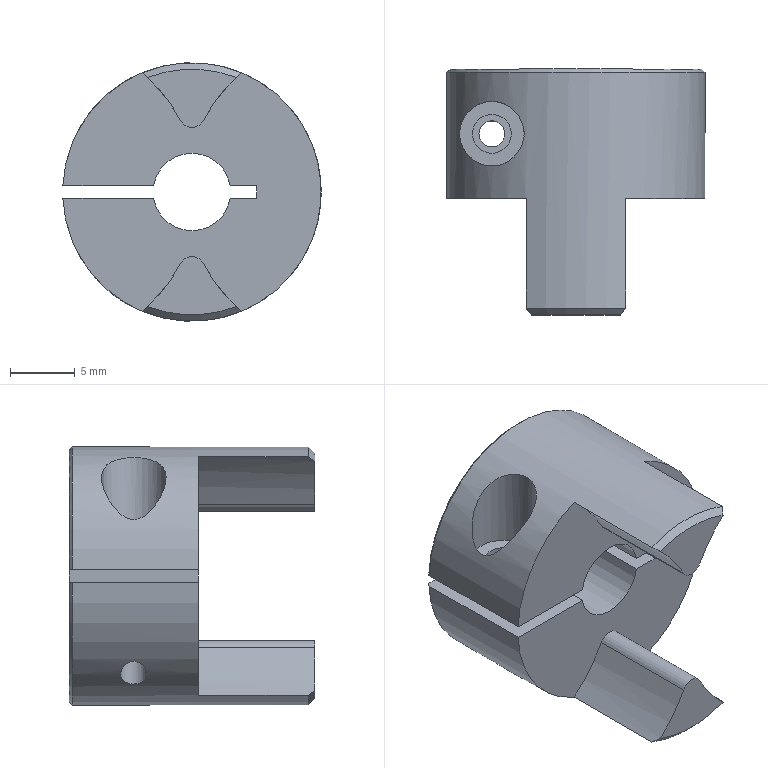Part | NX | features L-HUB_5003_022_GCJC20-BL-6-8 2 | 1 solid | 25 faces | box 19.987 x 19 x 20 mm | volume 3007 mm3 | cylinder 12 | plane 10 | cone 3 | commonest cylinder face diameters 24 x4 2 x2 6 x2 2.013 x1 3 x1 5 x1
STEP:
#1=CARTESIAN_POINT('',(-226.762,-568.6,-110.));
#2=VERTEX_POINT('',#1);
#3=CARTESIAN_POINT('',(-219.733,-568.6,-110.));
#4=VERTEX_POINT('',#3);
#5=CARTESIAN_POINT('',(-211.775,-568.6,-110.));
#6=DIRECTION('',(1.,0.,0.));
#7=VECTOR('',#6,1000.);
#8=LINE('',#5,#7);
#9=EDGE_CURVE('',#2,#4,#8,.T.);
#10=ORIENTED_EDGE('',*,*,#9,.T.);
#11=CARTESIAN_POINT('',(-213.817,-568.6,-110.));
#12=VERTEX_POINT('',#11);
#13=CARTESIAN_POINT('',(-216.775,-568.6,-110.5));
#14=DIRECTION('',(0.,1.,0.));
#15=DIRECTION('',(-1.,0.,0.));
#16=AXIS2_PLACEMENT_3D('',#13,#14,#15);
#17=CIRCLE('',#16,3.);
#18=EDGE_CURVE('',#4,#12,#17,.T.);
#19=ORIENTED_EDGE('',*,*,#18,.T.);
#20=CARTESIAN_POINT('',(-211.775,-568.6,-110.));
#21=VERTEX_POINT('',#20);
#22=CARTESIAN_POINT('',(-211.775,-568.6,-110.));
#23=DIRECTION('',(1.,0.,0.));
#24=VECTOR('',#23,1000.);
#25=LINE('',#22,#24);
#26=EDGE_CURVE('',#12,#21,#25,.T.);
#27=ORIENTED_EDGE('',*,*,#26,.T.);
#28=CARTESIAN_POINT('',(-211.775,-568.6,-111.));
#29=VERTEX_POINT('',#28);
#30=CARTESIAN_POINT('',(-211.775,-568.6,-111.));
#31=DIRECTION('',(0.,0.,-1.));
#32=VECTOR('',#31,1000.);
#33=LINE('',#30,#32);
#34=EDGE_CURVE('',#21,#29,#33,.T.);
#35=ORIENTED_EDGE('',*,*,#34,.T.);
#36=CARTESIAN_POINT('',(-213.817,-568.6,-111.));
#37=VERTEX_POINT('',#36);
#38=CARTESIAN_POINT('',(-226.762,-568.6,-111.));
#39=DIRECTION('',(-1.,0.,0.));
#40=VECTOR('',#39,1000.);
#41=LINE('',#38,#40);
#42=EDGE_CURVE('',#29,#37,#41,.T.);
#43=ORIENTED_EDGE('',*,*,#42,.T.);
#44=CARTESIAN_POINT('',(-219.733,-568.6,-111.));
#45=VERTEX_POINT('',#44);
#46=CARTESIAN_POINT('',(-216.775,-568.6,-110.5));
#47=DIRECTION('',(0.,1.,0.));
#48=DIRECTION('',(-1.,0.,0.));
#49=AXIS2_PLACEMENT_3D('',#46,#47,#48);
#50=CIRCLE('',#49,3.);
#51=EDGE_CURVE('',#37,#45,#50,.T.);
#52=ORIENTED_EDGE('',*,*,#51,.T.);
#53=CARTESIAN_POINT('',(-226.762,-568.6,-111.));
#54=VERTEX_POINT('',#53);
#55=CARTESIAN_POINT('',(-226.762,-568.6,-111.));
#56=DIRECTION('',(-1.,0.,0.));
#57=VECTOR('',#56,1000.);
#58=LINE('',#55,#57);
#59=EDGE_CURVE('',#45,#54,#58,.T.);
#60=ORIENTED_EDGE('',*,*,#59,.T.);
#61=CARTESIAN_POINT('',(-220.634,-568.6,-119.726));
#62=VERTEX_POINT('',#61);
#63=CARTESIAN_POINT('',(-216.775,-568.6,-110.5));
#64=DIRECTION('',(0.,1.,0.));
#65=DIRECTION('',(-1.,0.,0.));
#66=AXIS2_PLACEMENT_3D('',#63,#64,#65);
#67=CIRCLE('',#66,10.);
#68=EDGE_CURVE('',#62,#54,#67,.T.);
#69=ORIENTED_EDGE('',*,*,#68,.F.);
#70=CARTESIAN_POINT('',(-217.662,-568.6,-116.038));
#71=VERTEX_POINT('',#70);
#72=CARTESIAN_POINT('',(-228.308,-568.6,-110.5));
#73=DIRECTION('',(0.,1.,0.));
#74=DIRECTION('',(1.,0.,0.));
#75=AXIS2_PLACEMENT_3D('',#72,#73,#74);
#76=CIRCLE('',#75,12.);
#77=EDGE_CURVE('',#71,#62,#76,.T.);
#78=ORIENTED_EDGE('',*,*,#77,.F.);
#79=CARTESIAN_POINT('',(-215.888,-568.6,-116.038));
#80=VERTEX_POINT('',#79);
#81=CARTESIAN_POINT('',(-216.775,-568.6,-116.5));
#82=DIRECTION('',(0.,-1.,0.));
#83=DIRECTION('',(1.,0.,0.));
#84=AXIS2_PLACEMENT_3D('',#81,#82,#83);
#85=CIRCLE('',#84,1.);
#86=EDGE_CURVE('',#80,#71,#85,.T.);
#87=ORIENTED_EDGE('',*,*,#86,.F.);
#88=CARTESIAN_POINT('',(-212.916,-568.6,-119.726));
#89=VERTEX_POINT('',#88);
#90=CARTESIAN_POINT('',(-205.242,-568.6,-110.5));
#91=DIRECTION('',(0.,1.,0.));
#92=DIRECTION('',(1.,0.,0.));
#93=AXIS2_PLACEMENT_3D('',#90,#91,#92);
#94=CIRCLE('',#93,12.);
#95=EDGE_CURVE('',#89,#80,#94,.T.);
#96=ORIENTED_EDGE('',*,*,#95,.F.);
#97=CARTESIAN_POINT('',(-212.916,-568.6,-101.274));
#98=VERTEX_POINT('',#97);
#99=CARTESIAN_POINT('',(-216.775,-568.6,-110.5));
#100=DIRECTION('',(0.,1.,0.));
#101=DIRECTION('',(-1.,0.,0.));
#102=AXIS2_PLACEMENT_3D('',#99,#100,#101);
#103=CIRCLE('',#102,10.);
#104=EDGE_CURVE('',#98,#89,#103,.T.);
#105=ORIENTED_EDGE('',*,*,#104,.F.);
#106=CARTESIAN_POINT('',(-215.888,-568.6,-104.962));
#107=VERTEX_POINT('',#106);
#108=CARTESIAN_POINT('',(-205.242,-568.6,-110.5));
#109=DIRECTION('',(0.,1.,0.));
#110=DIRECTION('',(1.,0.,0.));
#111=AXIS2_PLACEMENT_3D('',#108,#109,#110);
#112=CIRCLE('',#111,12.);
#113=EDGE_CURVE('',#107,#98,#112,.T.);
#114=ORIENTED_EDGE('',*,*,#113,.F.);
#115=CARTESIAN_POINT('',(-217.662,-568.6,-104.962));
#116=VERTEX_POINT('',#115);
#117=CARTESIAN_POINT('',(-216.775,-568.6,-104.5));
#118=DIRECTION('',(0.,-1.,0.));
#119=DIRECTION('',(1.,0.,0.));
#120=AXIS2_PLACEMENT_3D('',#117,#118,#119);
#121=CIRCLE('',#120,1.);
#122=EDGE_CURVE('',#116,#107,#121,.T.);
#123=ORIENTED_EDGE('',*,*,#122,.F.);
#124=CARTESIAN_POINT('',(-220.634,-568.6,-101.274));
#125=VERTEX_POINT('',#124);
#126=CARTESIAN_POINT('',(-228.308,-568.6,-110.5));
#127=DIRECTION('',(0.,1.,0.));
#128=DIRECTION('',(1.,0.,0.));
#129=AXIS2_PLACEMENT_3D('',#126,#127,#128);
#130=CIRCLE('',#129,12.);
#131=EDGE_CURVE('',#125,#116,#130,.T.);
#132=ORIENTED_EDGE('',*,*,#131,.F.);
#133=CARTESIAN_POINT('',(-216.775,-568.6,-110.5));
#134=DIRECTION('',(0.,1.,0.));
#135=DIRECTION('',(-1.,0.,0.));
#136=AXIS2_PLACEMENT_3D('',#133,#134,#135);
#137=CIRCLE('',#136,10.);
#138=EDGE_CURVE('',#2,#125,#137,.T.);
#139=ORIENTED_EDGE('',*,*,#138,.F.);
#140=EDGE_LOOP('',(#10,#19,#27,#35,#43,#52,#60,#69,#78,#87,#96,#105,#114,#123,#132,#139));
#141=FACE_BOUND('',#140,.T.);
#142=CARTESIAN_POINT('',(-216.775,-568.6,-110.5));
#143=DIRECTION('',(0.,1.,0.));
#144=DIRECTION('',(-1.,0.,0.));
#145=AXIS2_PLACEMENT_3D('',#142,#143,#144);
#146=PLANE('',#145);
#147=ADVANCED_FACE('',(#141),#146,.F.);
#148=CARTESIAN_POINT('',(-219.733,-558.6,-110.));
#149=VERTEX_POINT('',#148);
#150=CARTESIAN_POINT('',(-226.512,-558.6,-110.));
#151=VERTEX_POINT('',#150);
#152=CARTESIAN_POINT('',(-211.775,-558.6,-110.));
#153=DIRECTION('',(-1.,0.,0.));
#154=VECTOR('',#153,1000.);
#155=LINE('',#152,#154);
#156=EDGE_CURVE('',#149,#151,#155,.T.);
#157=ORIENTED_EDGE('',*,*,#156,.T.);
#158=CARTESIAN_POINT('',(-226.512,-558.6,-111.));
#159=VERTEX_POINT('',#158);
#160=CARTESIAN_POINT('',(-216.775,-558.6,-110.5));
#161=DIRECTION('',(0.,-1.,0.));
#162=DIRECTION('',(1.,0.,0.));
#163=AXIS2_PLACEMENT_3D('',#160,#161,#162);
#164=CIRCLE('',#163,9.75);
#165=EDGE_CURVE('',#151,#159,#164,.F.);
#166=ORIENTED_EDGE('',*,*,#165,.T.);
#167=CARTESIAN_POINT('',(-219.733,-558.6,-111.));
#168=VERTEX_POINT('',#167);
#169=CARTESIAN_POINT('',(-226.762,-558.6,-111.));
#170=DIRECTION('',(1.,0.,0.));
#171=VECTOR('',#170,1000.);
#172=LINE('',#169,#171);
#173=EDGE_CURVE('',#159,#168,#172,.T.);
#174=ORIENTED_EDGE('',*,*,#173,.T.);
#175=CARTESIAN_POINT('',(-213.817,-558.6,-111.));
#176=VERTEX_POINT('',#175);
#177=CARTESIAN_POINT('',(-216.775,-558.6,-110.5));
#178=DIRECTION('',(0.,-1.,0.));
#179=DIRECTION('',(1.,0.,0.));
#180=AXIS2_PLACEMENT_3D('',#177,#178,#179);
#181=CIRCLE('',#180,3.);
#182=EDGE_CURVE('',#168,#176,#181,.T.);
#183=ORIENTED_EDGE('',*,*,#182,.T.);
#184=CARTESIAN_POINT('',(-211.775,-558.6,-111.));
#185=VERTEX_POINT('',#184);
#186=CARTESIAN_POINT('',(-226.762,-558.6,-111.));
#187=DIRECTION('',(1.,0.,0.));
#188=VECTOR('',#187,1000.);
#189=LINE('',#186,#188);
#190=EDGE_CURVE('',#176,#185,#189,.T.);
#191=ORIENTED_EDGE('',*,*,#190,.T.);
#192=CARTESIAN_POINT('',(-211.775,-558.6,-110.));
#193=VERTEX_POINT('',#192);
#194=CARTESIAN_POINT('',(-211.775,-558.6,-111.));
#195=DIRECTION('',(0.,0.,1.));
#196=VECTOR('',#195,1000.);
#197=LINE('',#194,#196);
#198=EDGE_CURVE('',#185,#193,#197,.T.);
#199=ORIENTED_EDGE('',*,*,#198,.T.);
#200=CARTESIAN_POINT('',(-213.817,-558.6,-110.));
#201=VERTEX_POINT('',#200);
#202=CARTESIAN_POINT('',(-211.775,-558.6,-110.));
#203=DIRECTION('',(-1.,0.,0.));
#204=VECTOR('',#203,1000.);
#205=LINE('',#202,#204);
#206=EDGE_CURVE('',#193,#201,#205,.T.);
#207=ORIENTED_EDGE('',*,*,#206,.T.);
#208=CARTESIAN_POINT('',(-216.775,-558.6,-110.5));
#209=DIRECTION('',(0.,-1.,0.));
#210=DIRECTION('',(1.,0.,0.));
#211=AXIS2_PLACEMENT_3D('',#208,#209,#210);
#212=CIRCLE('',#211,3.);
#213=EDGE_CURVE('',#201,#149,#212,.T.);
#214=ORIENTED_EDGE('',*,*,#213,.T.);
#215=EDGE_LOOP('',(#157,#166,#174,#183,#191,#199,#207,#214));
#216=FACE_BOUND('',#215,.T.);
#217=CARTESIAN_POINT('',(-216.775,-558.6,-110.5));
#218=DIRECTION('',(0.,-1.,0.));
#219=DIRECTION('',(1.,0.,0.));
#220=AXIS2_PLACEMENT_3D('',#217,#218,#219);
#221=PLANE('',#220);
#222=ADVANCED_FACE('',(#216),#221,.F.);
#223=CARTESIAN_POINT('',(-224.281,-563.6,-117.107));
#224=VERTEX_POINT('',#223);
#225=CARTESIAN_POINT('',(-223.988,-562.751,-117.443));
#226=CARTESIAN_POINT('',(-224.428,-563.601,-116.94));
#227=CARTESIAN_POINT('',(-223.989,-564.446,-117.441));
#228=CARTESIAN_POINT('',(-223.337,-564.673,-118.067));
#229=CARTESIAN_POINT('',(-222.587,-564.492,-118.651));
#230=CARTESIAN_POINT('',(-222.111,-563.607,-118.957));
#231=CARTESIAN_POINT('',(-222.58,-562.712,-118.656));
#232=CARTESIAN_POINT('',(-223.333,-562.526,-118.071));
#233=CARTESIAN_POINT('',(-223.988,-562.751,-117.443));
#234=CARTESIAN_POINT('',(-224.428,-563.601,-116.94));
#235=CARTESIAN_POINT('',(-223.989,-564.446,-117.441));
#236=B_SPLINE_CURVE_WITH_KNOTS('',3,(#225,#226,#227,#228,#229,#230,#231,#232,#233,#234,#235),.UNSPECIFIED.,.T.,.F.,(1,1,1,1,1,1,1,1,1,1,1,1,1,1,1),(-0.002758,-0.001839,-0.0009194,0.,0.0009194,0.001839,0.002758,0.003678,0.004597,0.005517,0.006436,0.007355,0.008275,0.009194,0.01011),.UNSPECIFIED.);
#237=EDGE_CURVE('',#224,#224,#236,.T.);
#238=ORIENTED_EDGE('',*,*,#237,.T.);
#239=EDGE_LOOP('',(#238));
#240=FACE_BOUND('',#239,.T.);
#241=CARTESIAN_POINT('',(-225.775,-563.6,-106.141));
#242=VERTEX_POINT('',#241);
#243=CARTESIAN_POINT('',(-225.578,-564.728,-105.73));
#244=CARTESIAN_POINT('',(-225.873,-563.6,-106.347));
#245=CARTESIAN_POINT('',(-225.579,-562.473,-105.73));
#246=CARTESIAN_POINT('',(-225.077,-561.81,-104.892));
#247=CARTESIAN_POINT('',(-224.42,-561.328,-104.023));
#248=CARTESIAN_POINT('',(-223.368,-560.991,-102.903));
#249=CARTESIAN_POINT('',(-221.65,-561.27,-101.683));
#250=CARTESIAN_POINT('',(-220.342,-563.585,-101.163));
#251=CARTESIAN_POINT('',(-221.632,-565.921,-101.673));
#252=CARTESIAN_POINT('',(-223.354,-566.211,-102.891));
#253=CARTESIAN_POINT('',(-224.415,-565.875,-104.017));
#254=CARTESIAN_POINT('',(-225.076,-565.391,-104.89));
#255=CARTESIAN_POINT('',(-225.578,-564.728,-105.73));
#256=CARTESIAN_POINT('',(-225.873,-563.6,-106.347));
#257=CARTESIAN_POINT('',(-225.579,-562.473,-105.73));
#258=B_SPLINE_CURVE_WITH_KNOTS('',3,(#243,#244,#245,#246,#247,#248,#249,#250,#251,#252,#253,#254,#255,#256,#257),.UNSPECIFIED.,.T.,.F.,(1,1,1,1,1,1,1,1,1,1,1,1,1,1,1,1,1,1,1),(-0.003565,-0.002377,-0.001188,0.,0.001188,0.002377,0.003565,0.004753,0.00713,0.009507,0.01188,0.01426,0.01545,0.01664,0.01783,0.01901,0.0202,0.02139,0.02258),.UNSPECIFIED.);
#259=EDGE_CURVE('',#242,#242,#258,.T.);
#260=ORIENTED_EDGE('',*,*,#259,.T.);
#261=EDGE_LOOP('',(#260));
#262=FACE_BOUND('',#261,.T.);
#263=CARTESIAN_POINT('',(-226.762,-558.85,-111.));
#264=VERTEX_POINT('',#263);
#265=CARTESIAN_POINT('',(-226.762,-583.633,-111.));
#266=DIRECTION('',(0.,1.,0.));
#267=VECTOR('',#266,1000.);
#268=LINE('',#265,#267);
#269=EDGE_CURVE('',#54,#264,#268,.T.);
#270=ORIENTED_EDGE('',*,*,#269,.T.);
#271=CARTESIAN_POINT('',(-226.762,-558.85,-110.));
#272=VERTEX_POINT('',#271);
#273=CARTESIAN_POINT('',(-216.775,-558.85,-110.5));
#274=DIRECTION('',(0.,-1.,0.));
#275=DIRECTION('',(1.,0.,0.));
#276=AXIS2_PLACEMENT_3D('',#273,#274,#275);
#277=CIRCLE('',#276,10.);
#278=EDGE_CURVE('',#264,#272,#277,.T.);
#279=ORIENTED_EDGE('',*,*,#278,.T.);
#280=CARTESIAN_POINT('',(-226.762,-583.633,-110.));
#281=DIRECTION('',(0.,1.,0.));
#282=VECTOR('',#281,1000.);
#283=LINE('',#280,#282);
#284=EDGE_CURVE('',#2,#272,#283,.T.);
#285=ORIENTED_EDGE('',*,*,#284,.F.);
#286=ORIENTED_EDGE('',*,*,#138,.T.);
#287=CARTESIAN_POINT('',(-220.634,-577.1,-101.274));
#288=VERTEX_POINT('',#287);
#289=CARTESIAN_POINT('',(-220.634,-577.6,-101.274));
#290=DIRECTION('',(0.,1.,0.));
#291=VECTOR('',#290,1000.);
#292=LINE('',#289,#291);
#293=EDGE_CURVE('',#288,#125,#292,.T.);
#294=ORIENTED_EDGE('',*,*,#293,.F.);
#295=CARTESIAN_POINT('',(-212.916,-577.1,-101.274));
#296=VERTEX_POINT('',#295);
#297=CARTESIAN_POINT('',(-216.775,-577.1,-110.5));
#298=DIRECTION('',(0.,-1.,0.));
#299=DIRECTION('',(1.,0.,0.));
#300=AXIS2_PLACEMENT_3D('',#297,#298,#299);
#301=CIRCLE('',#300,10.);
#302=EDGE_CURVE('',#288,#296,#301,.F.);
#303=ORIENTED_EDGE('',*,*,#302,.T.);
#304=CARTESIAN_POINT('',(-212.916,-577.6,-101.274));
#305=DIRECTION('',(0.,1.,0.));
#306=VECTOR('',#305,1000.);
#307=LINE('',#304,#306);
#308=EDGE_CURVE('',#296,#98,#307,.T.);
#309=ORIENTED_EDGE('',*,*,#308,.T.);
#310=ORIENTED_EDGE('',*,*,#104,.T.);
#311=CARTESIAN_POINT('',(-212.916,-577.1,-119.726));
#312=VERTEX_POINT('',#311);
#313=CARTESIAN_POINT('',(-212.916,-577.6,-119.726));
#314=DIRECTION('',(0.,1.,0.));
#315=VECTOR('',#314,1000.);
#316=LINE('',#313,#315);
#317=EDGE_CURVE('',#312,#89,#316,.T.);
#318=ORIENTED_EDGE('',*,*,#317,.F.);
#319=CARTESIAN_POINT('',(-220.634,-577.1,-119.726));
#320=VERTEX_POINT('',#319);
#321=CARTESIAN_POINT('',(-216.775,-577.1,-110.5));
#322=DIRECTION('',(0.,-1.,0.));
#323=DIRECTION('',(1.,0.,0.));
#324=AXIS2_PLACEMENT_3D('',#321,#322,#323);
#325=CIRCLE('',#324,10.);
#326=EDGE_CURVE('',#312,#320,#325,.F.);
#327=ORIENTED_EDGE('',*,*,#326,.T.);
#328=CARTESIAN_POINT('',(-220.634,-577.6,-119.726));
#329=DIRECTION('',(0.,1.,0.));
#330=VECTOR('',#329,1000.);
#331=LINE('',#328,#330);
#332=EDGE_CURVE('',#320,#62,#331,.T.);
#333=ORIENTED_EDGE('',*,*,#332,.T.);
#334=ORIENTED_EDGE('',*,*,#68,.T.);
#335=EDGE_LOOP('',(#270,#279,#285,#286,#294,#303,#309,#310,#318,#327,#333,#334));
#336=FACE_BOUND('',#335,.T.);
#337=CARTESIAN_POINT('',(-216.775,-557.65,-110.5));
#338=DIRECTION('',(0.,1.,0.));
#339=DIRECTION('',(-1.,0.,0.));
#340=AXIS2_PLACEMENT_3D('',#337,#338,#339);
#341=CYLINDRICAL_SURFACE('',#340,10.);
#342=ADVANCED_FACE('',(#240,#262,#336),#341,.T.);
#343=ORIENTED_EDGE('',*,*,#18,.F.);
#344=CARTESIAN_POINT('',(-219.733,-577.601,-110.));
#345=DIRECTION('',(0.,1.,0.));
#346=VECTOR('',#345,1000.);
#347=LINE('',#344,#346);
#348=EDGE_CURVE('',#4,#149,#347,.T.);
#349=ORIENTED_EDGE('',*,*,#348,.T.);
#350=ORIENTED_EDGE('',*,*,#213,.F.);
#351=CARTESIAN_POINT('',(-213.817,-577.601,-110.));
#352=DIRECTION('',(0.,1.,0.));
#353=VECTOR('',#352,1000.);
#354=LINE('',#351,#353);
#355=EDGE_CURVE('',#201,#12,#354,.F.);
#356=ORIENTED_EDGE('',*,*,#355,.T.);
#357=EDGE_LOOP('',(#343,#349,#350,#356));
#358=FACE_BOUND('',#357,.T.);
#359=CARTESIAN_POINT('',(-216.775,-577.601,-110.5));
#360=DIRECTION('',(0.,1.,0.));
#361=DIRECTION('',(-1.,0.,0.));
#362=AXIS2_PLACEMENT_3D('',#359,#360,#361);
#363=CYLINDRICAL_SURFACE('',#362,3.);
#364=ADVANCED_FACE('',(#358),#363,.F.);
#365=ORIENTED_EDGE('',*,*,#51,.F.);
#366=CARTESIAN_POINT('',(-213.817,-577.601,-111.));
#367=DIRECTION('',(0.,1.,0.));
#368=VECTOR('',#367,1000.);
#369=LINE('',#366,#368);
#370=EDGE_CURVE('',#37,#176,#369,.T.);
#371=ORIENTED_EDGE('',*,*,#370,.T.);
#372=ORIENTED_EDGE('',*,*,#182,.F.);
#373=CARTESIAN_POINT('',(-219.733,-577.601,-111.));
#374=DIRECTION('',(0.,1.,0.));
#375=VECTOR('',#374,1000.);
#376=LINE('',#373,#375);
#377=EDGE_CURVE('',#168,#45,#376,.F.);
#378=ORIENTED_EDGE('',*,*,#377,.T.);
#379=EDGE_LOOP('',(#365,#371,#372,#378));
#380=FACE_BOUND('',#379,.T.);
#381=CARTESIAN_POINT('',(-216.775,-577.601,-110.5));
#382=DIRECTION('',(0.,1.,0.));
#383=DIRECTION('',(-1.,0.,0.));
#384=AXIS2_PLACEMENT_3D('',#381,#382,#383);
#385=CYLINDRICAL_SURFACE('',#384,3.);
#386=ADVANCED_FACE('',(#380),#385,.F.);
#387=ORIENTED_EDGE('',*,*,#122,.T.);
#388=CARTESIAN_POINT('',(-215.888,-577.6,-104.962));
#389=VERTEX_POINT('',#388);
#390=CARTESIAN_POINT('',(-215.888,-577.6,-104.962));
#391=DIRECTION('',(0.,1.,0.));
#392=VECTOR('',#391,1000.);
#393=LINE('',#390,#392);
#394=EDGE_CURVE('',#389,#107,#393,.T.);
#395=ORIENTED_EDGE('',*,*,#394,.F.);
#396=CARTESIAN_POINT('',(-217.662,-577.6,-104.962));
#397=VERTEX_POINT('',#396);
#398=CARTESIAN_POINT('',(-216.775,-577.6,-104.5));
#399=DIRECTION('',(0.,-1.,0.));
#400=DIRECTION('',(1.,0.,0.));
#401=AXIS2_PLACEMENT_3D('',#398,#399,#400);
#402=CIRCLE('',#401,1.);
#403=EDGE_CURVE('',#397,#389,#402,.T.);
#404=ORIENTED_EDGE('',*,*,#403,.F.);
#405=CARTESIAN_POINT('',(-217.662,-577.6,-104.962));
#406=DIRECTION('',(0.,1.,0.));
#407=VECTOR('',#406,1000.);
#408=LINE('',#405,#407);
#409=EDGE_CURVE('',#397,#116,#408,.T.);
#410=ORIENTED_EDGE('',*,*,#409,.T.);
#411=EDGE_LOOP('',(#387,#395,#404,#410));
#412=FACE_BOUND('',#411,.T.);
#413=CARTESIAN_POINT('',(-216.775,-577.6,-104.5));
#414=DIRECTION('',(0.,1.,0.));
#415=DIRECTION('',(-1.,0.,0.));
#416=AXIS2_PLACEMENT_3D('',#413,#414,#415);
#417=CYLINDRICAL_SURFACE('',#416,1.);
#418=ADVANCED_FACE('',(#412),#417,.T.);
#419=ORIENTED_EDGE('',*,*,#308,.F.);
#420=CARTESIAN_POINT('',(-213.339,-577.6,-101.643));
#421=VERTEX_POINT('',#420);
#422=CARTESIAN_POINT('',(-212.916,-577.1,-101.274));
#423=CARTESIAN_POINT('',(-213.06,-577.266,-101.394));
#424=CARTESIAN_POINT('',(-213.201,-577.433,-101.517));
#425=CARTESIAN_POINT('',(-213.339,-577.6,-101.643));
#426=B_SPLINE_CURVE_WITH_KNOTS('',3,(#422,#423,#424,#425),.UNSPECIFIED.,.F.,.F.,(4,4),(0.,0.0007514),.UNSPECIFIED.);
#427=EDGE_CURVE('',#296,#421,#426,.T.);
#428=ORIENTED_EDGE('',*,*,#427,.T.);
#429=CARTESIAN_POINT('',(-205.242,-577.6,-110.5));
#430=DIRECTION('',(0.,1.,0.));
#431=DIRECTION('',(1.,0.,0.));
#432=AXIS2_PLACEMENT_3D('',#429,#430,#431);
#433=CIRCLE('',#432,12.);
#434=EDGE_CURVE('',#389,#421,#433,.T.);
#435=ORIENTED_EDGE('',*,*,#434,.F.);
#436=ORIENTED_EDGE('',*,*,#394,.T.);
#437=ORIENTED_EDGE('',*,*,#113,.T.);
#438=EDGE_LOOP('',(#419,#428,#435,#436,#437));
#439=FACE_BOUND('',#438,.T.);
#440=CARTESIAN_POINT('',(-205.242,-577.6,-110.5));
#441=DIRECTION('',(0.,1.,0.));
#442=DIRECTION('',(-1.,0.,0.));
#443=AXIS2_PLACEMENT_3D('',#440,#441,#442);
#444=CYLINDRICAL_SURFACE('',#443,12.);
#445=ADVANCED_FACE('',(#439),#444,.F.);
#446=CARTESIAN_POINT('',(-220.211,-577.6,-101.643));
#447=VERTEX_POINT('',#446);
#448=CARTESIAN_POINT('',(-228.308,-577.6,-110.5));
#449=DIRECTION('',(0.,1.,0.));
#450=DIRECTION('',(1.,0.,0.));
#451=AXIS2_PLACEMENT_3D('',#448,#449,#450);
#452=CIRCLE('',#451,12.);
#453=EDGE_CURVE('',#447,#397,#452,.T.);
#454=ORIENTED_EDGE('',*,*,#453,.F.);
#455=CARTESIAN_POINT('',(-220.211,-577.6,-101.643));
#456=CARTESIAN_POINT('',(-220.349,-577.433,-101.517));
#457=CARTESIAN_POINT('',(-220.49,-577.266,-101.394));
#458=CARTESIAN_POINT('',(-220.634,-577.1,-101.274));
#459=B_SPLINE_CURVE_WITH_KNOTS('',3,(#455,#456,#457,#458),.UNSPECIFIED.,.F.,.F.,(4,4),(0.,0.0007514),.UNSPECIFIED.);
#460=EDGE_CURVE('',#447,#288,#459,.T.);
#461=ORIENTED_EDGE('',*,*,#460,.T.);
#462=ORIENTED_EDGE('',*,*,#293,.T.);
#463=ORIENTED_EDGE('',*,*,#131,.T.);
#464=ORIENTED_EDGE('',*,*,#409,.F.);
#465=EDGE_LOOP('',(#454,#461,#462,#463,#464));
#466=FACE_BOUND('',#465,.T.);
#467=CARTESIAN_POINT('',(-228.308,-577.6,-110.5));
#468=DIRECTION('',(0.,1.,0.));
#469=DIRECTION('',(-1.,0.,0.));
#470=AXIS2_PLACEMENT_3D('',#467,#468,#469);
#471=CYLINDRICAL_SURFACE('',#470,12.);
#472=ADVANCED_FACE('',(#466),#471,.F.);
#473=ORIENTED_EDGE('',*,*,#434,.T.);
#474=CARTESIAN_POINT('',(-216.775,-577.6,-110.5));
#475=DIRECTION('',(0.,-1.,0.));
#476=DIRECTION('',(1.,0.,0.));
#477=AXIS2_PLACEMENT_3D('',#474,#475,#476);
#478=CIRCLE('',#477,9.5);
#479=EDGE_CURVE('',#421,#447,#478,.T.);
#480=ORIENTED_EDGE('',*,*,#479,.T.);
#481=ORIENTED_EDGE('',*,*,#453,.T.);
#482=ORIENTED_EDGE('',*,*,#403,.T.);
#483=EDGE_LOOP('',(#473,#480,#481,#482));
#484=FACE_BOUND('',#483,.T.);
#485=CARTESIAN_POINT('',(-211.009,-577.6,-107.5));
#486=DIRECTION('',(0.,-1.,0.));
#487=DIRECTION('',(1.,0.,0.));
#488=AXIS2_PLACEMENT_3D('',#485,#486,#487);
#489=PLANE('',#488);
#490=ADVANCED_FACE('',(#484),#489,.T.);
#491=ORIENTED_EDGE('',*,*,#86,.T.);
#492=CARTESIAN_POINT('',(-217.662,-577.6,-116.038));
#493=VERTEX_POINT('',#492);
#494=CARTESIAN_POINT('',(-217.662,-577.6,-116.038));
#495=DIRECTION('',(0.,1.,0.));
#496=VECTOR('',#495,1000.);
#497=LINE('',#494,#496);
#498=EDGE_CURVE('',#493,#71,#497,.T.);
#499=ORIENTED_EDGE('',*,*,#498,.F.);
#500=CARTESIAN_POINT('',(-215.888,-577.6,-116.038));
#501=VERTEX_POINT('',#500);
#502=CARTESIAN_POINT('',(-216.775,-577.6,-116.5));
#503=DIRECTION('',(0.,-1.,0.));
#504=DIRECTION('',(1.,0.,0.));
#505=AXIS2_PLACEMENT_3D('',#502,#503,#504);
#506=CIRCLE('',#505,1.);
#507=EDGE_CURVE('',#501,#493,#506,.T.);
#508=ORIENTED_EDGE('',*,*,#507,.F.);
#509=CARTESIAN_POINT('',(-215.888,-577.6,-116.038));
#510=DIRECTION('',(0.,1.,0.));
#511=VECTOR('',#510,1000.);
#512=LINE('',#509,#511);
#513=EDGE_CURVE('',#501,#80,#512,.T.);
#514=ORIENTED_EDGE('',*,*,#513,.T.);
#515=EDGE_LOOP('',(#491,#499,#508,#514));
#516=FACE_BOUND('',#515,.T.);
#517=CARTESIAN_POINT('',(-216.775,-577.6,-116.5));
#518=DIRECTION('',(0.,1.,0.));
#519=DIRECTION('',(-1.,0.,0.));
#520=AXIS2_PLACEMENT_3D('',#517,#518,#519);
#521=CYLINDRICAL_SURFACE('',#520,1.);
#522=ADVANCED_FACE('',(#516),#521,.T.);
#523=ORIENTED_EDGE('',*,*,#332,.F.);
#524=CARTESIAN_POINT('',(-220.211,-577.6,-119.357));
#525=VERTEX_POINT('',#524);
#526=CARTESIAN_POINT('',(-220.634,-577.1,-119.726));
#527=CARTESIAN_POINT('',(-220.49,-577.266,-119.606));
#528=CARTESIAN_POINT('',(-220.349,-577.433,-119.483));
#529=CARTESIAN_POINT('',(-220.211,-577.6,-119.357));
#530=B_SPLINE_CURVE_WITH_KNOTS('',3,(#526,#527,#528,#529),.UNSPECIFIED.,.F.,.F.,(4,4),(0.,0.0007514),.UNSPECIFIED.);
#531=EDGE_CURVE('',#320,#525,#530,.T.);
#532=ORIENTED_EDGE('',*,*,#531,.T.);
#533=CARTESIAN_POINT('',(-228.308,-577.6,-110.5));
#534=DIRECTION('',(0.,1.,0.));
#535=DIRECTION('',(1.,0.,0.));
#536=AXIS2_PLACEMENT_3D('',#533,#534,#535);
#537=CIRCLE('',#536,12.);
#538=EDGE_CURVE('',#493,#525,#537,.T.);
#539=ORIENTED_EDGE('',*,*,#538,.F.);
#540=ORIENTED_EDGE('',*,*,#498,.T.);
#541=ORIENTED_EDGE('',*,*,#77,.T.);
#542=EDGE_LOOP('',(#523,#532,#539,#540,#541));
#543=FACE_BOUND('',#542,.T.);
#544=CARTESIAN_POINT('',(-228.308,-577.6,-110.5));
#545=DIRECTION('',(0.,1.,0.));
#546=DIRECTION('',(-1.,0.,0.));
#547=AXIS2_PLACEMENT_3D('',#544,#545,#546);
#548=CYLINDRICAL_SURFACE('',#547,12.);
#549=ADVANCED_FACE('',(#543),#548,.F.);
#550=CARTESIAN_POINT('',(-213.339,-577.6,-119.357));
#551=VERTEX_POINT('',#550);
#552=CARTESIAN_POINT('',(-205.242,-577.6,-110.5));
#553=DIRECTION('',(0.,1.,0.));
#554=DIRECTION('',(1.,0.,0.));
#555=AXIS2_PLACEMENT_3D('',#552,#553,#554);
#556=CIRCLE('',#555,12.);
#557=EDGE_CURVE('',#551,#501,#556,.T.);
#558=ORIENTED_EDGE('',*,*,#557,.F.);
#559=CARTESIAN_POINT('',(-213.339,-577.6,-119.357));
#560=CARTESIAN_POINT('',(-213.201,-577.433,-119.483));
#561=CARTESIAN_POINT('',(-213.06,-577.266,-119.606));
#562=CARTESIAN_POINT('',(-212.916,-577.1,-119.726));
#563=B_SPLINE_CURVE_WITH_KNOTS('',3,(#559,#560,#561,#562),.UNSPECIFIED.,.F.,.F.,(4,4),(0.,0.0007514),.UNSPECIFIED.);
#564=EDGE_CURVE('',#551,#312,#563,.T.);
#565=ORIENTED_EDGE('',*,*,#564,.T.);
#566=ORIENTED_EDGE('',*,*,#317,.T.);
#567=ORIENTED_EDGE('',*,*,#95,.T.);
#568=ORIENTED_EDGE('',*,*,#513,.F.);
#569=EDGE_LOOP('',(#558,#565,#566,#567,#568));
#570=FACE_BOUND('',#569,.T.);
#571=CARTESIAN_POINT('',(-205.242,-577.6,-110.5));
#572=DIRECTION('',(0.,1.,0.));
#573=DIRECTION('',(-1.,0.,0.));
#574=AXIS2_PLACEMENT_3D('',#571,#572,#573);
#575=CYLINDRICAL_SURFACE('',#574,12.);
#576=ADVANCED_FACE('',(#570),#575,.F.);
#577=ORIENTED_EDGE('',*,*,#538,.T.);
#578=CARTESIAN_POINT('',(-216.775,-577.6,-110.5));
#579=DIRECTION('',(0.,-1.,0.));
#580=DIRECTION('',(1.,0.,0.));
#581=AXIS2_PLACEMENT_3D('',#578,#579,#580);
#582=CIRCLE('',#581,9.5);
#583=EDGE_CURVE('',#525,#551,#582,.T.);
#584=ORIENTED_EDGE('',*,*,#583,.T.);
#585=ORIENTED_EDGE('',*,*,#557,.T.);
#586=ORIENTED_EDGE('',*,*,#507,.T.);
#587=EDGE_LOOP('',(#577,#584,#585,#586));
#588=FACE_BOUND('',#587,.T.);
#589=CARTESIAN_POINT('',(-222.541,-577.6,-113.5));
#590=DIRECTION('',(0.,-1.,0.));
#591=DIRECTION('',(1.,0.,0.));
#592=AXIS2_PLACEMENT_3D('',#589,#590,#591);
#593=PLANE('',#592);
#594=ADVANCED_FACE('',(#588),#593,.T.);
#595=ORIENTED_EDGE('',*,*,#531,.F.);
#596=ORIENTED_EDGE('',*,*,#326,.F.);
#597=ORIENTED_EDGE('',*,*,#564,.F.);
#598=ORIENTED_EDGE('',*,*,#583,.F.);
#599=EDGE_LOOP('',(#595,#596,#597,#598));
#600=FACE_BOUND('',#599,.T.);
#601=CARTESIAN_POINT('',(-216.775,-577.6,-110.5));
#602=DIRECTION('',(0.,1.,0.));
#603=DIRECTION('',(-1.,0.,0.));
#604=AXIS2_PLACEMENT_3D('',#601,#602,#603);
#605=CONICAL_SURFACE('',#604,9.5,0.7854);
#606=ADVANCED_FACE('',(#600),#605,.T.);
#607=ORIENTED_EDGE('',*,*,#427,.F.);
#608=ORIENTED_EDGE('',*,*,#302,.F.);
#609=ORIENTED_EDGE('',*,*,#460,.F.);
#610=ORIENTED_EDGE('',*,*,#479,.F.);
#611=EDGE_LOOP('',(#607,#608,#609,#610));
#612=FACE_BOUND('',#611,.T.);
#613=CARTESIAN_POINT('',(-216.775,-577.6,-110.5));
#614=DIRECTION('',(0.,1.,0.));
#615=DIRECTION('',(-1.,0.,0.));
#616=AXIS2_PLACEMENT_3D('',#613,#614,#615);
#617=CONICAL_SURFACE('',#616,9.5,0.7854);
#618=ADVANCED_FACE('',(#612),#617,.T.);
#619=CARTESIAN_POINT('',(-224.281,-563.6,-111.));
#620=VERTEX_POINT('',#619);
#621=CARTESIAN_POINT('',(-223.275,-563.6,-111.));
#622=DIRECTION('',(0.,0.,1.));
#623=DIRECTION('',(-1.,0.,0.));
#624=AXIS2_PLACEMENT_3D('',#621,#622,#623);
#625=CIRCLE('',#624,1.006);
#626=EDGE_CURVE('',#620,#620,#625,.T.);
#627=ORIENTED_EDGE('',*,*,#626,.F.);
#628=EDGE_LOOP('',(#627));
#629=FACE_BOUND('',#628,.T.);
#630=ORIENTED_EDGE('',*,*,#173,.F.);
#631=CARTESIAN_POINT('',(-226.512,-558.6,-111.));
#632=CARTESIAN_POINT('',(-226.596,-558.683,-111.));
#633=CARTESIAN_POINT('',(-226.679,-558.767,-111.));
#634=CARTESIAN_POINT('',(-226.762,-558.85,-111.));
#635=B_SPLINE_CURVE_WITH_KNOTS('',3,(#631,#632,#633,#634),.UNSPECIFIED.,.F.,.F.,(4,4),(0.,0.0003538),.UNSPECIFIED.);
#636=EDGE_CURVE('',#159,#264,#635,.T.);
#637=ORIENTED_EDGE('',*,*,#636,.T.);
#638=ORIENTED_EDGE('',*,*,#269,.F.);
#639=ORIENTED_EDGE('',*,*,#59,.F.);
#640=ORIENTED_EDGE('',*,*,#377,.F.);
#641=EDGE_LOOP('',(#630,#637,#638,#639,#640));
#642=FACE_BOUND('',#641,.T.);
#643=CARTESIAN_POINT('',(-226.762,-583.633,-111.));
#644=DIRECTION('',(0.,0.,1.));
#645=DIRECTION('',(-1.,0.,0.));
#646=AXIS2_PLACEMENT_3D('',#643,#644,#645);
#647=PLANE('',#646);
#648=ADVANCED_FACE('',(#629,#642),#647,.T.);
#649=ORIENTED_EDGE('',*,*,#42,.F.);
#650=CARTESIAN_POINT('',(-211.775,-583.633,-111.));
#651=DIRECTION('',(0.,1.,0.));
#652=VECTOR('',#651,1000.);
#653=LINE('',#650,#652);
#654=EDGE_CURVE('',#29,#185,#653,.T.);
#655=ORIENTED_EDGE('',*,*,#654,.T.);
#656=ORIENTED_EDGE('',*,*,#190,.F.);
#657=ORIENTED_EDGE('',*,*,#370,.F.);
#658=EDGE_LOOP('',(#649,#655,#656,#657));
#659=FACE_BOUND('',#658,.T.);
#660=CARTESIAN_POINT('',(-226.762,-583.633,-111.));
#661=DIRECTION('',(0.,0.,1.));
#662=DIRECTION('',(-1.,0.,0.));
#663=AXIS2_PLACEMENT_3D('',#660,#661,#662);
#664=PLANE('',#663);
#665=ADVANCED_FACE('',(#659),#664,.T.);
#666=ORIENTED_EDGE('',*,*,#206,.F.);
#667=CARTESIAN_POINT('',(-211.775,-583.633,-110.));
#668=DIRECTION('',(0.,1.,0.));
#669=VECTOR('',#668,1000.);
#670=LINE('',#667,#669);
#671=EDGE_CURVE('',#21,#193,#670,.T.);
#672=ORIENTED_EDGE('',*,*,#671,.F.);
#673=ORIENTED_EDGE('',*,*,#26,.F.);
#674=ORIENTED_EDGE('',*,*,#355,.F.);
#675=EDGE_LOOP('',(#666,#672,#673,#674));
#676=FACE_BOUND('',#675,.T.);
#677=CARTESIAN_POINT('',(-211.775,-583.633,-110.));
#678=DIRECTION('',(0.,0.,-1.));
#679=DIRECTION('',(1.,0.,0.));
#680=AXIS2_PLACEMENT_3D('',#677,#678,#679);
#681=PLANE('',#680);
#682=ADVANCED_FACE('',(#676),#681,.T.);
#683=ORIENTED_EDGE('',*,*,#671,.T.);
#684=ORIENTED_EDGE('',*,*,#198,.F.);
#685=ORIENTED_EDGE('',*,*,#654,.F.);
#686=ORIENTED_EDGE('',*,*,#34,.F.);
#687=EDGE_LOOP('',(#683,#684,#685,#686));
#688=FACE_BOUND('',#687,.T.);
#689=CARTESIAN_POINT('',(-211.775,-583.633,-111.));
#690=DIRECTION('',(-1.,0.,0.));
#691=DIRECTION('',(0.,-1.,0.));
#692=AXIS2_PLACEMENT_3D('',#689,#690,#691);
#693=PLANE('',#692);
#694=ADVANCED_FACE('',(#688),#693,.T.);
#695=CARTESIAN_POINT('',(-221.775,-563.6,-110.));
#696=VERTEX_POINT('',#695);
#697=CARTESIAN_POINT('',(-223.275,-563.6,-110.));
#698=DIRECTION('',(0.,0.,-1.));
#699=DIRECTION('',(1.,0.,0.));
#700=AXIS2_PLACEMENT_3D('',#697,#698,#699);
#701=CIRCLE('',#700,1.5);
#702=EDGE_CURVE('',#696,#696,#701,.T.);
#703=ORIENTED_EDGE('',*,*,#702,.F.);
#704=EDGE_LOOP('',(#703));
#705=FACE_BOUND('',#704,.T.);
#706=ORIENTED_EDGE('',*,*,#284,.T.);
#707=CARTESIAN_POINT('',(-226.762,-558.85,-110.));
#708=CARTESIAN_POINT('',(-226.679,-558.767,-110.));
#709=CARTESIAN_POINT('',(-226.596,-558.683,-110.));
#710=CARTESIAN_POINT('',(-226.512,-558.6,-110.));
#711=B_SPLINE_CURVE_WITH_KNOTS('',3,(#707,#708,#709,#710),.UNSPECIFIED.,.F.,.F.,(4,4),(0.,0.0003538),.UNSPECIFIED.);
#712=EDGE_CURVE('',#272,#151,#711,.T.);
#713=ORIENTED_EDGE('',*,*,#712,.T.);
#714=ORIENTED_EDGE('',*,*,#156,.F.);
#715=ORIENTED_EDGE('',*,*,#348,.F.);
#716=ORIENTED_EDGE('',*,*,#9,.F.);
#717=EDGE_LOOP('',(#706,#713,#714,#715,#716));
#718=FACE_BOUND('',#717,.T.);
#719=CARTESIAN_POINT('',(-211.775,-583.633,-110.));
#720=DIRECTION('',(0.,0.,-1.));
#721=DIRECTION('',(1.,0.,0.));
#722=AXIS2_PLACEMENT_3D('',#719,#720,#721);
#723=PLANE('',#722);
#724=ADVANCED_FACE('',(#705,#718),#723,.T.);
#725=CARTESIAN_POINT('',(-225.775,-563.6,-107.8));
#726=VERTEX_POINT('',#725);
#727=CARTESIAN_POINT('',(-223.275,-563.6,-107.8));
#728=DIRECTION('',(0.,0.,1.));
#729=DIRECTION('',(-1.,0.,0.));
#730=AXIS2_PLACEMENT_3D('',#727,#728,#729);
#731=CIRCLE('',#730,2.5);
#732=EDGE_CURVE('',#726,#726,#731,.T.);
#733=ORIENTED_EDGE('',*,*,#732,.F.);
#734=EDGE_LOOP('',(#733));
#735=FACE_BOUND('',#734,.T.);
#736=ORIENTED_EDGE('',*,*,#259,.F.);
#737=EDGE_LOOP('',(#736));
#738=FACE_BOUND('',#737,.T.);
#739=CARTESIAN_POINT('',(-223.275,-563.6,-100.5));
#740=DIRECTION('',(0.,0.,1.));
#741=DIRECTION('',(-1.,0.,0.));
#742=AXIS2_PLACEMENT_3D('',#739,#740,#741);
#743=CYLINDRICAL_SURFACE('',#742,2.5);
#744=ADVANCED_FACE('',(#735,#738),#743,.F.);
#745=CARTESIAN_POINT('',(-224.775,-563.6,-107.8));
#746=VERTEX_POINT('',#745);
#747=CARTESIAN_POINT('',(-223.275,-563.6,-107.8));
#748=DIRECTION('',(0.,0.,1.));
#749=DIRECTION('',(-1.,0.,0.));
#750=AXIS2_PLACEMENT_3D('',#747,#748,#749);
#751=CIRCLE('',#750,1.5);
#752=EDGE_CURVE('',#746,#746,#751,.T.);
#753=ORIENTED_EDGE('',*,*,#752,.T.);
#754=EDGE_LOOP('',(#753));
#755=FACE_BOUND('',#754,.T.);
#756=ORIENTED_EDGE('',*,*,#702,.T.);
#757=EDGE_LOOP('',(#756));
#758=FACE_BOUND('',#757,.T.);
#759=CARTESIAN_POINT('',(-223.275,-563.6,-100.5));
#760=DIRECTION('',(0.,0.,1.));
#761=DIRECTION('',(-1.,0.,0.));
#762=AXIS2_PLACEMENT_3D('',#759,#760,#761);
#763=CYLINDRICAL_SURFACE('',#762,1.5);
#764=ADVANCED_FACE('',(#755,#758),#763,.F.);
#765=ORIENTED_EDGE('',*,*,#752,.F.);
#766=EDGE_LOOP('',(#765));
#767=FACE_BOUND('',#766,.T.);
#768=ORIENTED_EDGE('',*,*,#732,.T.);
#769=EDGE_LOOP('',(#768));
#770=FACE_BOUND('',#769,.T.);
#771=CARTESIAN_POINT('',(-223.275,-565.1,-107.8));
#772=DIRECTION('',(0.,0.,-1.));
#773=DIRECTION('',(1.,0.,0.));
#774=AXIS2_PLACEMENT_3D('',#771,#772,#773);
#775=PLANE('',#774);
#776=ADVANCED_FACE('',(#767,#770),#775,.F.);
#777=ORIENTED_EDGE('',*,*,#237,.F.);
#778=EDGE_LOOP('',(#777));
#779=FACE_BOUND('',#778,.T.);
#780=ORIENTED_EDGE('',*,*,#626,.T.);
#781=EDGE_LOOP('',(#780));
#782=FACE_BOUND('',#781,.T.);
#783=CARTESIAN_POINT('',(-223.275,-563.6,-111.));
#784=DIRECTION('',(0.,0.,1.));
#785=DIRECTION('',(-1.,0.,0.));
#786=AXIS2_PLACEMENT_3D('',#783,#784,#785);
#787=CYLINDRICAL_SURFACE('',#786,1.006);
#788=ADVANCED_FACE('',(#779,#782),#787,.F.);
#789=ORIENTED_EDGE('',*,*,#712,.F.);
#790=ORIENTED_EDGE('',*,*,#278,.F.);
#791=ORIENTED_EDGE('',*,*,#636,.F.);
#792=ORIENTED_EDGE('',*,*,#165,.F.);
#793=EDGE_LOOP('',(#789,#790,#791,#792));
#794=FACE_BOUND('',#793,.T.);
#795=CARTESIAN_POINT('',(-216.775,-558.6,-110.5));
#796=DIRECTION('',(0.,-1.,0.));
#797=DIRECTION('',(1.,0.,0.));
#798=AXIS2_PLACEMENT_3D('',#795,#796,#797);
#799=CONICAL_SURFACE('',#798,9.75,0.7854);
#800=ADVANCED_FACE('',(#794),#799,.T.);
#801=CLOSED_SHELL('',(#147,#222,#342,#364,#386,#418,#445,#472,#490,#522,#549,#576,#594,#606,#618,#648,#665,#682,#694,#724,#744,#764,#776,#788,#800));
#802=MANIFOLD_SOLID_BREP('',#801);
#803=(LENGTH_UNIT()NAMED_UNIT(*)SI_UNIT(.MILLI.,.METRE.));
#804=UNCERTAINTY_MEASURE_WITH_UNIT(LENGTH_MEASURE(0.0508),#803,'','');
#805=(NAMED_UNIT(*)PLANE_ANGLE_UNIT()SI_UNIT($,.RADIAN.));
#806=(NAMED_UNIT(*)SI_UNIT($,.STERADIAN.)SOLID_ANGLE_UNIT());
#807=(GEOMETRIC_REPRESENTATION_CONTEXT(3)GLOBAL_UNCERTAINTY_ASSIGNED_CONTEXT((#804))GLOBAL_UNIT_ASSIGNED_CONTEXT((#803,#805,#806))REPRESENTATION_CONTEXT('',''));
#808=ADVANCED_BREP_SHAPE_REPRESENTATION('',(#802),#807);